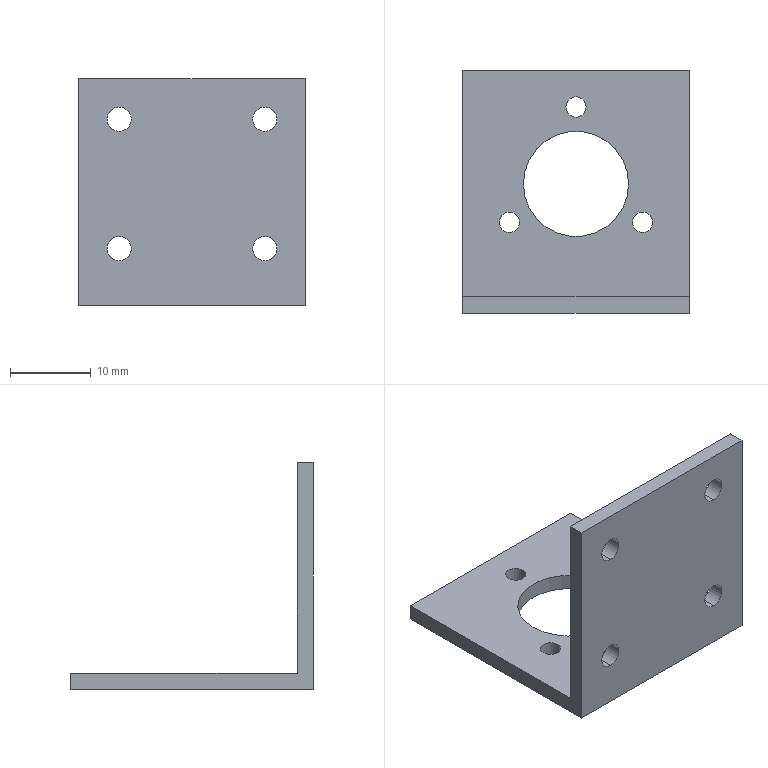Part | SolidWorks | features BaseBody 1 | 1 solid | 24 faces | box 28 x 30 x 28 mm | volume 2785 mm3 | cylinder 16 | plane 8 | commonest cylinder face diameters 3 x8 2.5 x6 13 x2
STEP:
#1=CARTESIAN_POINT('',(-9.,-16.,8.5));
#2=VERTEX_POINT('',#1);
#3=CARTESIAN_POINT('',(-9.,-16.,5.5));
#4=VERTEX_POINT('',#3);
#5=CARTESIAN_POINT('',(-9.,-16.,7.));
#6=DIRECTION('',(0.,-1.,0.));
#7=DIRECTION('',(0.,0.,1.));
#8=AXIS2_PLACEMENT_3D('',#5,#6,#7);
#9=CIRCLE('',#8,1.5);
#10=EDGE_CURVE('',#2,#4,#9,.T.);
#11=ORIENTED_EDGE('',*,*,#10,.T.);
#12=CARTESIAN_POINT('',(-9.,-14.,5.5));
#13=VERTEX_POINT('',#12);
#14=CARTESIAN_POINT('',(-9.,-24.,5.5));
#15=DIRECTION('',(0.,1.,0.));
#16=VECTOR('',#15,1000.);
#17=LINE('',#14,#16);
#18=EDGE_CURVE('',#4,#13,#17,.T.);
#19=ORIENTED_EDGE('',*,*,#18,.T.);
#20=CARTESIAN_POINT('',(-9.,-14.,8.5));
#21=VERTEX_POINT('',#20);
#22=CARTESIAN_POINT('',(-9.,-14.,7.));
#23=DIRECTION('',(0.,-1.,0.));
#24=DIRECTION('',(0.,0.,1.));
#25=AXIS2_PLACEMENT_3D('',#22,#23,#24);
#26=CIRCLE('',#25,1.5);
#27=EDGE_CURVE('',#21,#13,#26,.T.);
#28=ORIENTED_EDGE('',*,*,#27,.F.);
#29=CARTESIAN_POINT('',(-9.,-24.,8.5));
#30=DIRECTION('',(0.,1.,0.));
#31=VECTOR('',#30,1000.);
#32=LINE('',#29,#31);
#33=EDGE_CURVE('',#2,#21,#32,.T.);
#34=ORIENTED_EDGE('',*,*,#33,.F.);
#35=EDGE_LOOP('',(#11,#19,#28,#34));
#36=FACE_OUTER_BOUND('',#35,.T.);
#37=CARTESIAN_POINT('',(-9.,-24.,7.));
#38=DIRECTION('',(0.,1.,0.));
#39=DIRECTION('',(0.,0.,1.));
#40=AXIS2_PLACEMENT_3D('',#37,#38,#39);
#41=CYLINDRICAL_SURFACE('',#40,1.5);
#42=ADVANCED_FACE('',(#36),#41,.F.);
#43=CARTESIAN_POINT('',(-9.,-16.,24.5));
#44=VERTEX_POINT('',#43);
#45=CARTESIAN_POINT('',(-9.,-16.,21.5));
#46=VERTEX_POINT('',#45);
#47=CARTESIAN_POINT('',(-9.,-16.,23.));
#48=DIRECTION('',(0.,-1.,0.));
#49=DIRECTION('',(0.,0.,1.));
#50=AXIS2_PLACEMENT_3D('',#47,#48,#49);
#51=CIRCLE('',#50,1.5);
#52=EDGE_CURVE('',#44,#46,#51,.T.);
#53=ORIENTED_EDGE('',*,*,#52,.T.);
#54=CARTESIAN_POINT('',(-9.,-14.,21.5));
#55=VERTEX_POINT('',#54);
#56=CARTESIAN_POINT('',(-9.,-24.,21.5));
#57=DIRECTION('',(0.,1.,0.));
#58=VECTOR('',#57,1000.);
#59=LINE('',#56,#58);
#60=EDGE_CURVE('',#46,#55,#59,.T.);
#61=ORIENTED_EDGE('',*,*,#60,.T.);
#62=CARTESIAN_POINT('',(-9.,-14.,24.5));
#63=VERTEX_POINT('',#62);
#64=CARTESIAN_POINT('',(-9.,-14.,23.));
#65=DIRECTION('',(0.,-1.,0.));
#66=DIRECTION('',(0.,0.,1.));
#67=AXIS2_PLACEMENT_3D('',#64,#65,#66);
#68=CIRCLE('',#67,1.5);
#69=EDGE_CURVE('',#63,#55,#68,.T.);
#70=ORIENTED_EDGE('',*,*,#69,.F.);
#71=CARTESIAN_POINT('',(-9.,-24.,24.5));
#72=DIRECTION('',(0.,1.,0.));
#73=VECTOR('',#72,1000.);
#74=LINE('',#71,#73);
#75=EDGE_CURVE('',#44,#63,#74,.T.);
#76=ORIENTED_EDGE('',*,*,#75,.F.);
#77=EDGE_LOOP('',(#53,#61,#70,#76));
#78=FACE_OUTER_BOUND('',#77,.T.);
#79=CARTESIAN_POINT('',(-9.,-24.,23.));
#80=DIRECTION('',(0.,1.,0.));
#81=DIRECTION('',(0.,0.,1.));
#82=AXIS2_PLACEMENT_3D('',#79,#80,#81);
#83=CYLINDRICAL_SURFACE('',#82,1.5);
#84=ADVANCED_FACE('',(#78),#83,.F.);
#85=CARTESIAN_POINT('',(9.,-16.,24.5));
#86=VERTEX_POINT('',#85);
#87=CARTESIAN_POINT('',(9.,-16.,21.5));
#88=VERTEX_POINT('',#87);
#89=CARTESIAN_POINT('',(9.,-16.,23.));
#90=DIRECTION('',(0.,-1.,0.));
#91=DIRECTION('',(0.,0.,1.));
#92=AXIS2_PLACEMENT_3D('',#89,#90,#91);
#93=CIRCLE('',#92,1.5);
#94=EDGE_CURVE('',#86,#88,#93,.T.);
#95=ORIENTED_EDGE('',*,*,#94,.T.);
#96=CARTESIAN_POINT('',(9.,-14.,21.5));
#97=VERTEX_POINT('',#96);
#98=CARTESIAN_POINT('',(9.,-24.,21.5));
#99=DIRECTION('',(0.,1.,0.));
#100=VECTOR('',#99,1000.);
#101=LINE('',#98,#100);
#102=EDGE_CURVE('',#88,#97,#101,.T.);
#103=ORIENTED_EDGE('',*,*,#102,.T.);
#104=CARTESIAN_POINT('',(9.,-14.,24.5));
#105=VERTEX_POINT('',#104);
#106=CARTESIAN_POINT('',(9.,-14.,23.));
#107=DIRECTION('',(0.,-1.,0.));
#108=DIRECTION('',(0.,0.,1.));
#109=AXIS2_PLACEMENT_3D('',#106,#107,#108);
#110=CIRCLE('',#109,1.5);
#111=EDGE_CURVE('',#105,#97,#110,.T.);
#112=ORIENTED_EDGE('',*,*,#111,.F.);
#113=CARTESIAN_POINT('',(9.,-24.,24.5));
#114=DIRECTION('',(0.,1.,0.));
#115=VECTOR('',#114,1000.);
#116=LINE('',#113,#115);
#117=EDGE_CURVE('',#86,#105,#116,.T.);
#118=ORIENTED_EDGE('',*,*,#117,.F.);
#119=EDGE_LOOP('',(#95,#103,#112,#118));
#120=FACE_OUTER_BOUND('',#119,.T.);
#121=CARTESIAN_POINT('',(9.,-24.,23.));
#122=DIRECTION('',(0.,1.,0.));
#123=DIRECTION('',(0.,0.,1.));
#124=AXIS2_PLACEMENT_3D('',#121,#122,#123);
#125=CYLINDRICAL_SURFACE('',#124,1.5);
#126=ADVANCED_FACE('',(#120),#125,.F.);
#127=CARTESIAN_POINT('',(9.,-16.,8.5));
#128=VERTEX_POINT('',#127);
#129=CARTESIAN_POINT('',(9.,-16.,5.5));
#130=VERTEX_POINT('',#129);
#131=CARTESIAN_POINT('',(9.,-16.,7.));
#132=DIRECTION('',(0.,-1.,0.));
#133=DIRECTION('',(0.,0.,1.));
#134=AXIS2_PLACEMENT_3D('',#131,#132,#133);
#135=CIRCLE('',#134,1.5);
#136=EDGE_CURVE('',#128,#130,#135,.T.);
#137=ORIENTED_EDGE('',*,*,#136,.T.);
#138=CARTESIAN_POINT('',(9.,-14.,5.5));
#139=VERTEX_POINT('',#138);
#140=CARTESIAN_POINT('',(9.,-24.,5.5));
#141=DIRECTION('',(0.,1.,0.));
#142=VECTOR('',#141,1000.);
#143=LINE('',#140,#142);
#144=EDGE_CURVE('',#130,#139,#143,.T.);
#145=ORIENTED_EDGE('',*,*,#144,.T.);
#146=CARTESIAN_POINT('',(9.,-14.,8.5));
#147=VERTEX_POINT('',#146);
#148=CARTESIAN_POINT('',(9.,-14.,7.));
#149=DIRECTION('',(0.,-1.,0.));
#150=DIRECTION('',(0.,0.,1.));
#151=AXIS2_PLACEMENT_3D('',#148,#149,#150);
#152=CIRCLE('',#151,1.5);
#153=EDGE_CURVE('',#147,#139,#152,.T.);
#154=ORIENTED_EDGE('',*,*,#153,.F.);
#155=CARTESIAN_POINT('',(9.,-24.,8.5));
#156=DIRECTION('',(0.,1.,0.));
#157=VECTOR('',#156,1000.);
#158=LINE('',#155,#157);
#159=EDGE_CURVE('',#128,#147,#158,.T.);
#160=ORIENTED_EDGE('',*,*,#159,.F.);
#161=EDGE_LOOP('',(#137,#145,#154,#160));
#162=FACE_OUTER_BOUND('',#161,.T.);
#163=CARTESIAN_POINT('',(9.,-24.,7.));
#164=DIRECTION('',(0.,1.,0.));
#165=DIRECTION('',(0.,0.,1.));
#166=AXIS2_PLACEMENT_3D('',#163,#164,#165);
#167=CYLINDRICAL_SURFACE('',#166,1.5);
#168=ADVANCED_FACE('',(#162),#167,.F.);
#169=CARTESIAN_POINT('',(-6.977,-4.75,0.));
#170=VERTEX_POINT('',#169);
#171=CARTESIAN_POINT('',(-9.477,-4.75,0.));
#172=VERTEX_POINT('',#171);
#173=CARTESIAN_POINT('',(-8.227,-4.75,0.));
#174=DIRECTION('',(0.,0.,-1.));
#175=DIRECTION('',(1.,0.,0.));
#176=AXIS2_PLACEMENT_3D('',#173,#174,#175);
#177=CIRCLE('',#176,1.25);
#178=EDGE_CURVE('',#170,#172,#177,.T.);
#179=ORIENTED_EDGE('',*,*,#178,.T.);
#180=CARTESIAN_POINT('',(-9.477,-4.75,2.));
#181=VERTEX_POINT('',#180);
#182=CARTESIAN_POINT('',(-9.477,-4.75,0.));
#183=DIRECTION('',(0.,0.,1.));
#184=VECTOR('',#183,1000.);
#185=LINE('',#182,#184);
#186=EDGE_CURVE('',#172,#181,#185,.T.);
#187=ORIENTED_EDGE('',*,*,#186,.T.);
#188=CARTESIAN_POINT('',(-6.977,-4.75,2.));
#189=VERTEX_POINT('',#188);
#190=CARTESIAN_POINT('',(-8.227,-4.75,2.));
#191=DIRECTION('',(0.,0.,-1.));
#192=DIRECTION('',(1.,0.,0.));
#193=AXIS2_PLACEMENT_3D('',#190,#191,#192);
#194=CIRCLE('',#193,1.25);
#195=EDGE_CURVE('',#189,#181,#194,.T.);
#196=ORIENTED_EDGE('',*,*,#195,.F.);
#197=CARTESIAN_POINT('',(-6.977,-4.75,0.));
#198=DIRECTION('',(0.,0.,1.));
#199=VECTOR('',#198,1000.);
#200=LINE('',#197,#199);
#201=EDGE_CURVE('',#170,#189,#200,.T.);
#202=ORIENTED_EDGE('',*,*,#201,.F.);
#203=EDGE_LOOP('',(#179,#187,#196,#202));
#204=FACE_OUTER_BOUND('',#203,.T.);
#205=CARTESIAN_POINT('',(-8.227,-4.75,0.));
#206=DIRECTION('',(0.,0.,1.));
#207=DIRECTION('',(1.,0.,0.));
#208=AXIS2_PLACEMENT_3D('',#205,#206,#207);
#209=CYLINDRICAL_SURFACE('',#208,1.25);
#210=ADVANCED_FACE('',(#204),#209,.F.);
#211=CARTESIAN_POINT('',(9.477,-4.75,0.));
#212=VERTEX_POINT('',#211);
#213=CARTESIAN_POINT('',(6.977,-4.75,0.));
#214=VERTEX_POINT('',#213);
#215=CARTESIAN_POINT('',(8.227,-4.75,0.));
#216=DIRECTION('',(0.,0.,-1.));
#217=DIRECTION('',(1.,0.,0.));
#218=AXIS2_PLACEMENT_3D('',#215,#216,#217);
#219=CIRCLE('',#218,1.25);
#220=EDGE_CURVE('',#212,#214,#219,.T.);
#221=ORIENTED_EDGE('',*,*,#220,.T.);
#222=CARTESIAN_POINT('',(6.977,-4.75,2.));
#223=VERTEX_POINT('',#222);
#224=CARTESIAN_POINT('',(6.977,-4.75,0.));
#225=DIRECTION('',(0.,0.,1.));
#226=VECTOR('',#225,1000.);
#227=LINE('',#224,#226);
#228=EDGE_CURVE('',#214,#223,#227,.T.);
#229=ORIENTED_EDGE('',*,*,#228,.T.);
#230=CARTESIAN_POINT('',(9.477,-4.75,2.));
#231=VERTEX_POINT('',#230);
#232=CARTESIAN_POINT('',(8.227,-4.75,2.));
#233=DIRECTION('',(0.,0.,-1.));
#234=DIRECTION('',(1.,0.,0.));
#235=AXIS2_PLACEMENT_3D('',#232,#233,#234);
#236=CIRCLE('',#235,1.25);
#237=EDGE_CURVE('',#231,#223,#236,.T.);
#238=ORIENTED_EDGE('',*,*,#237,.F.);
#239=CARTESIAN_POINT('',(9.477,-4.75,0.));
#240=DIRECTION('',(0.,0.,1.));
#241=VECTOR('',#240,1000.);
#242=LINE('',#239,#241);
#243=EDGE_CURVE('',#212,#231,#242,.T.);
#244=ORIENTED_EDGE('',*,*,#243,.F.);
#245=EDGE_LOOP('',(#221,#229,#238,#244));
#246=FACE_OUTER_BOUND('',#245,.T.);
#247=CARTESIAN_POINT('',(8.227,-4.75,0.));
#248=DIRECTION('',(0.,0.,1.));
#249=DIRECTION('',(1.,0.,0.));
#250=AXIS2_PLACEMENT_3D('',#247,#248,#249);
#251=CYLINDRICAL_SURFACE('',#250,1.25);
#252=ADVANCED_FACE('',(#246),#251,.F.);
#253=CARTESIAN_POINT('',(6.5,0.,0.));
#254=VERTEX_POINT('',#253);
#255=CARTESIAN_POINT('',(-6.5,0.,0.));
#256=VERTEX_POINT('',#255);
#257=CARTESIAN_POINT('',(0.,0.,0.));
#258=DIRECTION('',(0.,0.,-1.));
#259=DIRECTION('',(1.,0.,0.));
#260=AXIS2_PLACEMENT_3D('',#257,#258,#259);
#261=CIRCLE('',#260,6.5);
#262=EDGE_CURVE('',#254,#256,#261,.T.);
#263=ORIENTED_EDGE('',*,*,#262,.T.);
#264=CARTESIAN_POINT('',(-6.5,0.,2.));
#265=VERTEX_POINT('',#264);
#266=CARTESIAN_POINT('',(-6.5,0.,0.));
#267=DIRECTION('',(0.,0.,1.));
#268=VECTOR('',#267,1000.);
#269=LINE('',#266,#268);
#270=EDGE_CURVE('',#256,#265,#269,.T.);
#271=ORIENTED_EDGE('',*,*,#270,.T.);
#272=CARTESIAN_POINT('',(6.5,0.,2.));
#273=VERTEX_POINT('',#272);
#274=CARTESIAN_POINT('',(0.,0.,2.));
#275=DIRECTION('',(0.,0.,-1.));
#276=DIRECTION('',(1.,0.,0.));
#277=AXIS2_PLACEMENT_3D('',#274,#275,#276);
#278=CIRCLE('',#277,6.5);
#279=EDGE_CURVE('',#273,#265,#278,.T.);
#280=ORIENTED_EDGE('',*,*,#279,.F.);
#281=CARTESIAN_POINT('',(6.5,0.,0.));
#282=DIRECTION('',(0.,0.,1.));
#283=VECTOR('',#282,1000.);
#284=LINE('',#281,#283);
#285=EDGE_CURVE('',#254,#273,#284,.T.);
#286=ORIENTED_EDGE('',*,*,#285,.F.);
#287=EDGE_LOOP('',(#263,#271,#280,#286));
#288=FACE_OUTER_BOUND('',#287,.T.);
#289=CARTESIAN_POINT('',(0.,0.,0.));
#290=DIRECTION('',(0.,0.,1.));
#291=DIRECTION('',(1.,0.,0.));
#292=AXIS2_PLACEMENT_3D('',#289,#290,#291);
#293=CYLINDRICAL_SURFACE('',#292,6.5);
#294=ADVANCED_FACE('',(#288),#293,.F.);
#295=CARTESIAN_POINT('',(1.25,9.5,0.));
#296=VERTEX_POINT('',#295);
#297=CARTESIAN_POINT('',(-1.25,9.5,0.));
#298=VERTEX_POINT('',#297);
#299=CARTESIAN_POINT('',(0.,9.5,0.));
#300=DIRECTION('',(0.,0.,-1.));
#301=DIRECTION('',(1.,0.,0.));
#302=AXIS2_PLACEMENT_3D('',#299,#300,#301);
#303=CIRCLE('',#302,1.25);
#304=EDGE_CURVE('',#296,#298,#303,.T.);
#305=ORIENTED_EDGE('',*,*,#304,.T.);
#306=CARTESIAN_POINT('',(-1.25,9.5,2.));
#307=VERTEX_POINT('',#306);
#308=CARTESIAN_POINT('',(-1.25,9.5,0.));
#309=DIRECTION('',(0.,0.,1.));
#310=VECTOR('',#309,1000.);
#311=LINE('',#308,#310);
#312=EDGE_CURVE('',#298,#307,#311,.T.);
#313=ORIENTED_EDGE('',*,*,#312,.T.);
#314=CARTESIAN_POINT('',(1.25,9.5,2.));
#315=VERTEX_POINT('',#314);
#316=CARTESIAN_POINT('',(0.,9.5,2.));
#317=DIRECTION('',(0.,0.,-1.));
#318=DIRECTION('',(1.,0.,0.));
#319=AXIS2_PLACEMENT_3D('',#316,#317,#318);
#320=CIRCLE('',#319,1.25);
#321=EDGE_CURVE('',#315,#307,#320,.T.);
#322=ORIENTED_EDGE('',*,*,#321,.F.);
#323=CARTESIAN_POINT('',(1.25,9.5,0.));
#324=DIRECTION('',(0.,0.,1.));
#325=VECTOR('',#324,1000.);
#326=LINE('',#323,#325);
#327=EDGE_CURVE('',#296,#315,#326,.T.);
#328=ORIENTED_EDGE('',*,*,#327,.F.);
#329=EDGE_LOOP('',(#305,#313,#322,#328));
#330=FACE_OUTER_BOUND('',#329,.T.);
#331=CARTESIAN_POINT('',(0.,9.5,0.));
#332=DIRECTION('',(0.,0.,1.));
#333=DIRECTION('',(1.,0.,0.));
#334=AXIS2_PLACEMENT_3D('',#331,#332,#333);
#335=CYLINDRICAL_SURFACE('',#334,1.25);
#336=ADVANCED_FACE('',(#330),#335,.F.);
#337=CARTESIAN_POINT('',(14.,-16.,28.));
#338=VERTEX_POINT('',#337);
#339=CARTESIAN_POINT('',(14.,-16.,0.));
#340=VERTEX_POINT('',#339);
#341=CARTESIAN_POINT('',(14.,-16.,0.));
#342=DIRECTION('',(0.,0.,-1.));
#343=VECTOR('',#342,1000.);
#344=LINE('',#341,#343);
#345=EDGE_CURVE('',#338,#340,#344,.T.);
#346=ORIENTED_EDGE('',*,*,#345,.F.);
#347=CARTESIAN_POINT('',(-14.,-16.,28.));
#348=VERTEX_POINT('',#347);
#349=CARTESIAN_POINT('',(0.,-16.,28.));
#350=DIRECTION('',(1.,0.,0.));
#351=VECTOR('',#350,1000.);
#352=LINE('',#349,#351);
#353=EDGE_CURVE('',#348,#338,#352,.T.);
#354=ORIENTED_EDGE('',*,*,#353,.F.);
#355=CARTESIAN_POINT('',(-14.,-16.,0.));
#356=VERTEX_POINT('',#355);
#357=CARTESIAN_POINT('',(-14.,-16.,0.));
#358=DIRECTION('',(0.,0.,1.));
#359=VECTOR('',#358,1000.);
#360=LINE('',#357,#359);
#361=EDGE_CURVE('',#356,#348,#360,.T.);
#362=ORIENTED_EDGE('',*,*,#361,.F.);
#363=CARTESIAN_POINT('',(0.,-16.,0.));
#364=DIRECTION('',(-1.,0.,0.));
#365=VECTOR('',#364,1000.);
#366=LINE('',#363,#365);
#367=EDGE_CURVE('',#340,#356,#366,.T.);
#368=ORIENTED_EDGE('',*,*,#367,.F.);
#369=EDGE_LOOP('',(#346,#354,#362,#368));
#370=FACE_OUTER_BOUND('',#369,.T.);
#371=ORIENTED_EDGE('',*,*,#10,.F.);
#372=CARTESIAN_POINT('',(-9.,-16.,7.));
#373=DIRECTION('',(0.,-1.,0.));
#374=DIRECTION('',(0.,0.,1.));
#375=AXIS2_PLACEMENT_3D('',#372,#373,#374);
#376=CIRCLE('',#375,1.5);
#377=EDGE_CURVE('',#4,#2,#376,.T.);
#378=ORIENTED_EDGE('',*,*,#377,.F.);
#379=EDGE_LOOP('',(#371,#378));
#380=FACE_BOUND('',#379,.T.);
#381=ORIENTED_EDGE('',*,*,#52,.F.);
#382=CARTESIAN_POINT('',(-9.,-16.,23.));
#383=DIRECTION('',(0.,-1.,0.));
#384=DIRECTION('',(0.,0.,1.));
#385=AXIS2_PLACEMENT_3D('',#382,#383,#384);
#386=CIRCLE('',#385,1.5);
#387=EDGE_CURVE('',#46,#44,#386,.T.);
#388=ORIENTED_EDGE('',*,*,#387,.F.);
#389=EDGE_LOOP('',(#381,#388));
#390=FACE_BOUND('',#389,.T.);
#391=ORIENTED_EDGE('',*,*,#94,.F.);
#392=CARTESIAN_POINT('',(9.,-16.,23.));
#393=DIRECTION('',(0.,-1.,0.));
#394=DIRECTION('',(0.,0.,1.));
#395=AXIS2_PLACEMENT_3D('',#392,#393,#394);
#396=CIRCLE('',#395,1.5);
#397=EDGE_CURVE('',#88,#86,#396,.T.);
#398=ORIENTED_EDGE('',*,*,#397,.F.);
#399=EDGE_LOOP('',(#391,#398));
#400=FACE_BOUND('',#399,.T.);
#401=ORIENTED_EDGE('',*,*,#136,.F.);
#402=CARTESIAN_POINT('',(9.,-16.,7.));
#403=DIRECTION('',(0.,-1.,0.));
#404=DIRECTION('',(0.,0.,1.));
#405=AXIS2_PLACEMENT_3D('',#402,#403,#404);
#406=CIRCLE('',#405,1.5);
#407=EDGE_CURVE('',#130,#128,#406,.T.);
#408=ORIENTED_EDGE('',*,*,#407,.F.);
#409=EDGE_LOOP('',(#401,#408));
#410=FACE_BOUND('',#409,.T.);
#411=CARTESIAN_POINT('',(0.,-16.,0.));
#412=DIRECTION('',(0.,1.,0.));
#413=DIRECTION('',(0.,0.,1.));
#414=AXIS2_PLACEMENT_3D('',#411,#412,#413);
#415=PLANE('',#414);
#416=ADVANCED_FACE('',(#370,#380,#390,#400,#410),#415,.F.);
#417=ORIENTED_EDGE('',*,*,#367,.T.);
#418=CARTESIAN_POINT('',(-14.,14.,0.));
#419=VERTEX_POINT('',#418);
#420=CARTESIAN_POINT('',(-14.,0.,0.));
#421=DIRECTION('',(0.,-1.,0.));
#422=VECTOR('',#421,1000.);
#423=LINE('',#420,#422);
#424=EDGE_CURVE('',#419,#356,#423,.T.);
#425=ORIENTED_EDGE('',*,*,#424,.F.);
#426=CARTESIAN_POINT('',(14.,14.,0.));
#427=VERTEX_POINT('',#426);
#428=CARTESIAN_POINT('',(0.,14.,0.));
#429=DIRECTION('',(-1.,0.,0.));
#430=VECTOR('',#429,1000.);
#431=LINE('',#428,#430);
#432=EDGE_CURVE('',#427,#419,#431,.T.);
#433=ORIENTED_EDGE('',*,*,#432,.F.);
#434=CARTESIAN_POINT('',(14.,0.,0.));
#435=DIRECTION('',(0.,1.,0.));
#436=VECTOR('',#435,1000.);
#437=LINE('',#434,#436);
#438=EDGE_CURVE('',#340,#427,#437,.T.);
#439=ORIENTED_EDGE('',*,*,#438,.F.);
#440=EDGE_LOOP('',(#417,#425,#433,#439));
#441=FACE_OUTER_BOUND('',#440,.T.);
#442=ORIENTED_EDGE('',*,*,#178,.F.);
#443=CARTESIAN_POINT('',(-8.227,-4.75,0.));
#444=DIRECTION('',(0.,0.,-1.));
#445=DIRECTION('',(1.,0.,0.));
#446=AXIS2_PLACEMENT_3D('',#443,#444,#445);
#447=CIRCLE('',#446,1.25);
#448=EDGE_CURVE('',#172,#170,#447,.T.);
#449=ORIENTED_EDGE('',*,*,#448,.F.);
#450=EDGE_LOOP('',(#442,#449));
#451=FACE_BOUND('',#450,.T.);
#452=ORIENTED_EDGE('',*,*,#220,.F.);
#453=CARTESIAN_POINT('',(8.227,-4.75,0.));
#454=DIRECTION('',(0.,0.,-1.));
#455=DIRECTION('',(1.,0.,0.));
#456=AXIS2_PLACEMENT_3D('',#453,#454,#455);
#457=CIRCLE('',#456,1.25);
#458=EDGE_CURVE('',#214,#212,#457,.T.);
#459=ORIENTED_EDGE('',*,*,#458,.F.);
#460=EDGE_LOOP('',(#452,#459));
#461=FACE_BOUND('',#460,.T.);
#462=ORIENTED_EDGE('',*,*,#262,.F.);
#463=CARTESIAN_POINT('',(0.,0.,0.));
#464=DIRECTION('',(0.,0.,-1.));
#465=DIRECTION('',(1.,0.,0.));
#466=AXIS2_PLACEMENT_3D('',#463,#464,#465);
#467=CIRCLE('',#466,6.5);
#468=EDGE_CURVE('',#256,#254,#467,.T.);
#469=ORIENTED_EDGE('',*,*,#468,.F.);
#470=EDGE_LOOP('',(#462,#469));
#471=FACE_BOUND('',#470,.T.);
#472=ORIENTED_EDGE('',*,*,#304,.F.);
#473=CARTESIAN_POINT('',(0.,9.5,0.));
#474=DIRECTION('',(0.,0.,-1.));
#475=DIRECTION('',(1.,0.,0.));
#476=AXIS2_PLACEMENT_3D('',#473,#474,#475);
#477=CIRCLE('',#476,1.25);
#478=EDGE_CURVE('',#298,#296,#477,.T.);
#479=ORIENTED_EDGE('',*,*,#478,.F.);
#480=EDGE_LOOP('',(#472,#479));
#481=FACE_BOUND('',#480,.T.);
#482=CARTESIAN_POINT('',(0.,0.,0.));
#483=DIRECTION('',(0.,0.,1.));
#484=DIRECTION('',(1.,0.,0.));
#485=AXIS2_PLACEMENT_3D('',#482,#483,#484);
#486=PLANE('',#485);
#487=ADVANCED_FACE('',(#441,#451,#461,#471,#481),#486,.F.);
#488=CARTESIAN_POINT('',(14.,14.,2.));
#489=VERTEX_POINT('',#488);
#490=CARTESIAN_POINT('',(14.,14.,2.));
#491=DIRECTION('',(0.,0.,-1.));
#492=VECTOR('',#491,1000.);
#493=LINE('',#490,#492);
#494=EDGE_CURVE('',#489,#427,#493,.T.);
#495=ORIENTED_EDGE('',*,*,#494,.F.);
#496=CARTESIAN_POINT('',(14.,-14.,2.));
#497=VERTEX_POINT('',#496);
#498=CARTESIAN_POINT('',(14.,14.,2.));
#499=DIRECTION('',(0.,1.,0.));
#500=VECTOR('',#499,1000.);
#501=LINE('',#498,#500);
#502=EDGE_CURVE('',#497,#489,#501,.T.);
#503=ORIENTED_EDGE('',*,*,#502,.F.);
#504=CARTESIAN_POINT('',(14.,-14.,28.));
#505=VERTEX_POINT('',#504);
#506=CARTESIAN_POINT('',(14.,-14.,2.));
#507=DIRECTION('',(0.,0.,-1.));
#508=VECTOR('',#507,1000.);
#509=LINE('',#506,#508);
#510=EDGE_CURVE('',#505,#497,#509,.T.);
#511=ORIENTED_EDGE('',*,*,#510,.F.);
#512=CARTESIAN_POINT('',(14.,14.,28.));
#513=DIRECTION('',(0.,1.,0.));
#514=VECTOR('',#513,1000.);
#515=LINE('',#512,#514);
#516=EDGE_CURVE('',#338,#505,#515,.T.);
#517=ORIENTED_EDGE('',*,*,#516,.F.);
#518=ORIENTED_EDGE('',*,*,#345,.T.);
#519=ORIENTED_EDGE('',*,*,#438,.T.);
#520=EDGE_LOOP('',(#495,#503,#511,#517,#518,#519));
#521=FACE_OUTER_BOUND('',#520,.T.);
#522=CARTESIAN_POINT('',(14.,14.,2.));
#523=DIRECTION('',(-1.,0.,0.));
#524=DIRECTION('',(0.,-1.,0.));
#525=AXIS2_PLACEMENT_3D('',#522,#523,#524);
#526=PLANE('',#525);
#527=ADVANCED_FACE('',(#521),#526,.F.);
#528=CARTESIAN_POINT('',(-14.,-14.,28.));
#529=VERTEX_POINT('',#528);
#530=CARTESIAN_POINT('',(-14.,-16.,28.));
#531=DIRECTION('',(0.,1.,0.));
#532=VECTOR('',#531,1000.);
#533=LINE('',#530,#532);
#534=EDGE_CURVE('',#348,#529,#533,.T.);
#535=ORIENTED_EDGE('',*,*,#534,.F.);
#536=ORIENTED_EDGE('',*,*,#353,.T.);
#537=ORIENTED_EDGE('',*,*,#516,.T.);
#538=CARTESIAN_POINT('',(-14.,-14.,28.));
#539=DIRECTION('',(1.,0.,0.));
#540=VECTOR('',#539,1000.);
#541=LINE('',#538,#540);
#542=EDGE_CURVE('',#529,#505,#541,.T.);
#543=ORIENTED_EDGE('',*,*,#542,.F.);
#544=EDGE_LOOP('',(#535,#536,#537,#543));
#545=FACE_OUTER_BOUND('',#544,.T.);
#546=CARTESIAN_POINT('',(-14.,-16.,28.));
#547=DIRECTION('',(0.,0.,-1.));
#548=DIRECTION('',(-1.,0.,0.));
#549=AXIS2_PLACEMENT_3D('',#546,#547,#548);
#550=PLANE('',#549);
#551=ADVANCED_FACE('',(#545),#550,.F.);
#552=ORIENTED_EDGE('',*,*,#361,.T.);
#553=ORIENTED_EDGE('',*,*,#534,.T.);
#554=CARTESIAN_POINT('',(-14.,-14.,2.));
#555=VERTEX_POINT('',#554);
#556=CARTESIAN_POINT('',(-14.,-14.,2.));
#557=DIRECTION('',(0.,0.,1.));
#558=VECTOR('',#557,1000.);
#559=LINE('',#556,#558);
#560=EDGE_CURVE('',#555,#529,#559,.T.);
#561=ORIENTED_EDGE('',*,*,#560,.F.);
#562=CARTESIAN_POINT('',(-14.,14.,2.));
#563=VERTEX_POINT('',#562);
#564=CARTESIAN_POINT('',(-14.,14.,2.));
#565=DIRECTION('',(0.,-1.,0.));
#566=VECTOR('',#565,1000.);
#567=LINE('',#564,#566);
#568=EDGE_CURVE('',#563,#555,#567,.T.);
#569=ORIENTED_EDGE('',*,*,#568,.F.);
#570=CARTESIAN_POINT('',(-14.,14.,2.));
#571=DIRECTION('',(0.,0.,1.));
#572=VECTOR('',#571,1000.);
#573=LINE('',#570,#572);
#574=EDGE_CURVE('',#419,#563,#573,.T.);
#575=ORIENTED_EDGE('',*,*,#574,.F.);
#576=ORIENTED_EDGE('',*,*,#424,.T.);
#577=EDGE_LOOP('',(#552,#553,#561,#569,#575,#576));
#578=FACE_OUTER_BOUND('',#577,.T.);
#579=CARTESIAN_POINT('',(-14.,14.,2.));
#580=DIRECTION('',(1.,0.,0.));
#581=DIRECTION('',(0.,1.,0.));
#582=AXIS2_PLACEMENT_3D('',#579,#580,#581);
#583=PLANE('',#582);
#584=ADVANCED_FACE('',(#578),#583,.F.);
#585=ORIENTED_EDGE('',*,*,#18,.F.);
#586=ORIENTED_EDGE('',*,*,#377,.T.);
#587=ORIENTED_EDGE('',*,*,#33,.T.);
#588=CARTESIAN_POINT('',(-9.,-14.,7.));
#589=DIRECTION('',(0.,-1.,0.));
#590=DIRECTION('',(0.,0.,1.));
#591=AXIS2_PLACEMENT_3D('',#588,#589,#590);
#592=CIRCLE('',#591,1.5);
#593=EDGE_CURVE('',#13,#21,#592,.T.);
#594=ORIENTED_EDGE('',*,*,#593,.F.);
#595=EDGE_LOOP('',(#585,#586,#587,#594));
#596=FACE_OUTER_BOUND('',#595,.T.);
#597=CARTESIAN_POINT('',(-9.,-24.,7.));
#598=DIRECTION('',(0.,1.,0.));
#599=DIRECTION('',(0.,0.,1.));
#600=AXIS2_PLACEMENT_3D('',#597,#598,#599);
#601=CYLINDRICAL_SURFACE('',#600,1.5);
#602=ADVANCED_FACE('',(#596),#601,.F.);
#603=ORIENTED_EDGE('',*,*,#60,.F.);
#604=ORIENTED_EDGE('',*,*,#387,.T.);
#605=ORIENTED_EDGE('',*,*,#75,.T.);
#606=CARTESIAN_POINT('',(-9.,-14.,23.));
#607=DIRECTION('',(0.,-1.,0.));
#608=DIRECTION('',(0.,0.,1.));
#609=AXIS2_PLACEMENT_3D('',#606,#607,#608);
#610=CIRCLE('',#609,1.5);
#611=EDGE_CURVE('',#55,#63,#610,.T.);
#612=ORIENTED_EDGE('',*,*,#611,.F.);
#613=EDGE_LOOP('',(#603,#604,#605,#612));
#614=FACE_OUTER_BOUND('',#613,.T.);
#615=CARTESIAN_POINT('',(-9.,-24.,23.));
#616=DIRECTION('',(0.,1.,0.));
#617=DIRECTION('',(0.,0.,1.));
#618=AXIS2_PLACEMENT_3D('',#615,#616,#617);
#619=CYLINDRICAL_SURFACE('',#618,1.5);
#620=ADVANCED_FACE('',(#614),#619,.F.);
#621=ORIENTED_EDGE('',*,*,#102,.F.);
#622=ORIENTED_EDGE('',*,*,#397,.T.);
#623=ORIENTED_EDGE('',*,*,#117,.T.);
#624=CARTESIAN_POINT('',(9.,-14.,23.));
#625=DIRECTION('',(0.,-1.,0.));
#626=DIRECTION('',(0.,0.,1.));
#627=AXIS2_PLACEMENT_3D('',#624,#625,#626);
#628=CIRCLE('',#627,1.5);
#629=EDGE_CURVE('',#97,#105,#628,.T.);
#630=ORIENTED_EDGE('',*,*,#629,.F.);
#631=EDGE_LOOP('',(#621,#622,#623,#630));
#632=FACE_OUTER_BOUND('',#631,.T.);
#633=CARTESIAN_POINT('',(9.,-24.,23.));
#634=DIRECTION('',(0.,1.,0.));
#635=DIRECTION('',(0.,0.,1.));
#636=AXIS2_PLACEMENT_3D('',#633,#634,#635);
#637=CYLINDRICAL_SURFACE('',#636,1.5);
#638=ADVANCED_FACE('',(#632),#637,.F.);
#639=ORIENTED_EDGE('',*,*,#144,.F.);
#640=ORIENTED_EDGE('',*,*,#407,.T.);
#641=ORIENTED_EDGE('',*,*,#159,.T.);
#642=CARTESIAN_POINT('',(9.,-14.,7.));
#643=DIRECTION('',(0.,-1.,0.));
#644=DIRECTION('',(0.,0.,1.));
#645=AXIS2_PLACEMENT_3D('',#642,#643,#644);
#646=CIRCLE('',#645,1.5);
#647=EDGE_CURVE('',#139,#147,#646,.T.);
#648=ORIENTED_EDGE('',*,*,#647,.F.);
#649=EDGE_LOOP('',(#639,#640,#641,#648));
#650=FACE_OUTER_BOUND('',#649,.T.);
#651=CARTESIAN_POINT('',(9.,-24.,7.));
#652=DIRECTION('',(0.,1.,0.));
#653=DIRECTION('',(0.,0.,1.));
#654=AXIS2_PLACEMENT_3D('',#651,#652,#653);
#655=CYLINDRICAL_SURFACE('',#654,1.5);
#656=ADVANCED_FACE('',(#650),#655,.F.);
#657=ORIENTED_EDGE('',*,*,#574,.T.);
#658=CARTESIAN_POINT('',(-14.,14.,2.));
#659=DIRECTION('',(-1.,0.,0.));
#660=VECTOR('',#659,1000.);
#661=LINE('',#658,#660);
#662=EDGE_CURVE('',#489,#563,#661,.T.);
#663=ORIENTED_EDGE('',*,*,#662,.F.);
#664=ORIENTED_EDGE('',*,*,#494,.T.);
#665=ORIENTED_EDGE('',*,*,#432,.T.);
#666=EDGE_LOOP('',(#657,#663,#664,#665));
#667=FACE_OUTER_BOUND('',#666,.T.);
#668=CARTESIAN_POINT('',(-14.,14.,2.));
#669=DIRECTION('',(0.,-1.,0.));
#670=DIRECTION('',(0.,0.,-1.));
#671=AXIS2_PLACEMENT_3D('',#668,#669,#670);
#672=PLANE('',#671);
#673=ADVANCED_FACE('',(#667),#672,.F.);
#674=ORIENTED_EDGE('',*,*,#186,.F.);
#675=ORIENTED_EDGE('',*,*,#448,.T.);
#676=ORIENTED_EDGE('',*,*,#201,.T.);
#677=CARTESIAN_POINT('',(-8.227,-4.75,2.));
#678=DIRECTION('',(0.,0.,-1.));
#679=DIRECTION('',(1.,0.,0.));
#680=AXIS2_PLACEMENT_3D('',#677,#678,#679);
#681=CIRCLE('',#680,1.25);
#682=EDGE_CURVE('',#181,#189,#681,.T.);
#683=ORIENTED_EDGE('',*,*,#682,.F.);
#684=EDGE_LOOP('',(#674,#675,#676,#683));
#685=FACE_OUTER_BOUND('',#684,.T.);
#686=CARTESIAN_POINT('',(-8.227,-4.75,0.));
#687=DIRECTION('',(0.,0.,1.));
#688=DIRECTION('',(1.,0.,0.));
#689=AXIS2_PLACEMENT_3D('',#686,#687,#688);
#690=CYLINDRICAL_SURFACE('',#689,1.25);
#691=ADVANCED_FACE('',(#685),#690,.F.);
#692=ORIENTED_EDGE('',*,*,#228,.F.);
#693=ORIENTED_EDGE('',*,*,#458,.T.);
#694=ORIENTED_EDGE('',*,*,#243,.T.);
#695=CARTESIAN_POINT('',(8.227,-4.75,2.));
#696=DIRECTION('',(0.,0.,-1.));
#697=DIRECTION('',(1.,0.,0.));
#698=AXIS2_PLACEMENT_3D('',#695,#696,#697);
#699=CIRCLE('',#698,1.25);
#700=EDGE_CURVE('',#223,#231,#699,.T.);
#701=ORIENTED_EDGE('',*,*,#700,.F.);
#702=EDGE_LOOP('',(#692,#693,#694,#701));
#703=FACE_OUTER_BOUND('',#702,.T.);
#704=CARTESIAN_POINT('',(8.227,-4.75,0.));
#705=DIRECTION('',(0.,0.,1.));
#706=DIRECTION('',(1.,0.,0.));
#707=AXIS2_PLACEMENT_3D('',#704,#705,#706);
#708=CYLINDRICAL_SURFACE('',#707,1.25);
#709=ADVANCED_FACE('',(#703),#708,.F.);
#710=ORIENTED_EDGE('',*,*,#270,.F.);
#711=ORIENTED_EDGE('',*,*,#468,.T.);
#712=ORIENTED_EDGE('',*,*,#285,.T.);
#713=CARTESIAN_POINT('',(0.,0.,2.));
#714=DIRECTION('',(0.,0.,-1.));
#715=DIRECTION('',(1.,0.,0.));
#716=AXIS2_PLACEMENT_3D('',#713,#714,#715);
#717=CIRCLE('',#716,6.5);
#718=EDGE_CURVE('',#265,#273,#717,.T.);
#719=ORIENTED_EDGE('',*,*,#718,.F.);
#720=EDGE_LOOP('',(#710,#711,#712,#719));
#721=FACE_OUTER_BOUND('',#720,.T.);
#722=CARTESIAN_POINT('',(0.,0.,0.));
#723=DIRECTION('',(0.,0.,1.));
#724=DIRECTION('',(1.,0.,0.));
#725=AXIS2_PLACEMENT_3D('',#722,#723,#724);
#726=CYLINDRICAL_SURFACE('',#725,6.5);
#727=ADVANCED_FACE('',(#721),#726,.F.);
#728=ORIENTED_EDGE('',*,*,#312,.F.);
#729=ORIENTED_EDGE('',*,*,#478,.T.);
#730=ORIENTED_EDGE('',*,*,#327,.T.);
#731=CARTESIAN_POINT('',(0.,9.5,2.));
#732=DIRECTION('',(0.,0.,-1.));
#733=DIRECTION('',(1.,0.,0.));
#734=AXIS2_PLACEMENT_3D('',#731,#732,#733);
#735=CIRCLE('',#734,1.25);
#736=EDGE_CURVE('',#307,#315,#735,.T.);
#737=ORIENTED_EDGE('',*,*,#736,.F.);
#738=EDGE_LOOP('',(#728,#729,#730,#737));
#739=FACE_OUTER_BOUND('',#738,.T.);
#740=CARTESIAN_POINT('',(0.,9.5,0.));
#741=DIRECTION('',(0.,0.,1.));
#742=DIRECTION('',(1.,0.,0.));
#743=AXIS2_PLACEMENT_3D('',#740,#741,#742);
#744=CYLINDRICAL_SURFACE('',#743,1.25);
#745=ADVANCED_FACE('',(#739),#744,.F.);
#746=ORIENTED_EDGE('',*,*,#568,.T.);
#747=CARTESIAN_POINT('',(0.,-14.,2.));
#748=DIRECTION('',(1.,0.,0.));
#749=VECTOR('',#748,1000.);
#750=LINE('',#747,#749);
#751=EDGE_CURVE('',#555,#497,#750,.T.);
#752=ORIENTED_EDGE('',*,*,#751,.T.);
#753=ORIENTED_EDGE('',*,*,#502,.T.);
#754=ORIENTED_EDGE('',*,*,#662,.T.);
#755=EDGE_LOOP('',(#746,#752,#753,#754));
#756=FACE_OUTER_BOUND('',#755,.T.);
#757=ORIENTED_EDGE('',*,*,#195,.T.);
#758=ORIENTED_EDGE('',*,*,#682,.T.);
#759=EDGE_LOOP('',(#757,#758));
#760=FACE_BOUND('',#759,.T.);
#761=ORIENTED_EDGE('',*,*,#237,.T.);
#762=ORIENTED_EDGE('',*,*,#700,.T.);
#763=EDGE_LOOP('',(#761,#762));
#764=FACE_BOUND('',#763,.T.);
#765=ORIENTED_EDGE('',*,*,#279,.T.);
#766=ORIENTED_EDGE('',*,*,#718,.T.);
#767=EDGE_LOOP('',(#765,#766));
#768=FACE_BOUND('',#767,.T.);
#769=ORIENTED_EDGE('',*,*,#321,.T.);
#770=ORIENTED_EDGE('',*,*,#736,.T.);
#771=EDGE_LOOP('',(#769,#770));
#772=FACE_BOUND('',#771,.T.);
#773=CARTESIAN_POINT('',(0.,0.,2.));
#774=DIRECTION('',(0.,0.,1.));
#775=DIRECTION('',(1.,0.,0.));
#776=AXIS2_PLACEMENT_3D('',#773,#774,#775);
#777=PLANE('',#776);
#778=ADVANCED_FACE('',(#756,#760,#764,#768,#772),#777,.T.);
#779=ORIENTED_EDGE('',*,*,#542,.T.);
#780=ORIENTED_EDGE('',*,*,#510,.T.);
#781=ORIENTED_EDGE('',*,*,#751,.F.);
#782=ORIENTED_EDGE('',*,*,#560,.T.);
#783=EDGE_LOOP('',(#779,#780,#781,#782));
#784=FACE_OUTER_BOUND('',#783,.T.);
#785=ORIENTED_EDGE('',*,*,#27,.T.);
#786=ORIENTED_EDGE('',*,*,#593,.T.);
#787=EDGE_LOOP('',(#785,#786));
#788=FACE_BOUND('',#787,.T.);
#789=ORIENTED_EDGE('',*,*,#69,.T.);
#790=ORIENTED_EDGE('',*,*,#611,.T.);
#791=EDGE_LOOP('',(#789,#790));
#792=FACE_BOUND('',#791,.T.);
#793=ORIENTED_EDGE('',*,*,#111,.T.);
#794=ORIENTED_EDGE('',*,*,#629,.T.);
#795=EDGE_LOOP('',(#793,#794));
#796=FACE_BOUND('',#795,.T.);
#797=ORIENTED_EDGE('',*,*,#153,.T.);
#798=ORIENTED_EDGE('',*,*,#647,.T.);
#799=EDGE_LOOP('',(#797,#798));
#800=FACE_BOUND('',#799,.T.);
#801=CARTESIAN_POINT('',(0.,-14.,0.));
#802=DIRECTION('',(0.,1.,0.));
#803=DIRECTION('',(0.,0.,1.));
#804=AXIS2_PLACEMENT_3D('',#801,#802,#803);
#805=PLANE('',#804);
#806=ADVANCED_FACE('',(#784,#788,#792,#796,#800),#805,.T.);
#807=CLOSED_SHELL('',(#42,#84,#126,#168,#210,#252,#294,#336,#416,#487,#527,#551,#584,#602,#620,#638,#656,#673,#691,#709,#727,#745,#778,#806));
#808=MANIFOLD_SOLID_BREP('',#807);
#809=CARTESIAN_POINT('',(0.,0.,0.));
#810=DIRECTION('',(0.,0.,1.));
#811=DIRECTION('',(1.,0.,0.));
#812=AXIS2_PLACEMENT_3D('',#809,#810,#811);
#813=(LENGTH_UNIT()NAMED_UNIT(*)SI_UNIT(.MILLI.,.METRE.));
#814=UNCERTAINTY_MEASURE_WITH_UNIT(LENGTH_MEASURE(0.00001),#813,'','');
#815=(NAMED_UNIT(*)PLANE_ANGLE_UNIT()SI_UNIT($,.RADIAN.));
#816=(NAMED_UNIT(*)SI_UNIT($,.STERADIAN.)SOLID_ANGLE_UNIT());
#817=(GEOMETRIC_REPRESENTATION_CONTEXT(3)GLOBAL_UNCERTAINTY_ASSIGNED_CONTEXT((#814))GLOBAL_UNIT_ASSIGNED_CONTEXT((#813,#815,#816))REPRESENTATION_CONTEXT('',''));
#818=ADVANCED_BREP_SHAPE_REPRESENTATION('',(#808,#812),#817);